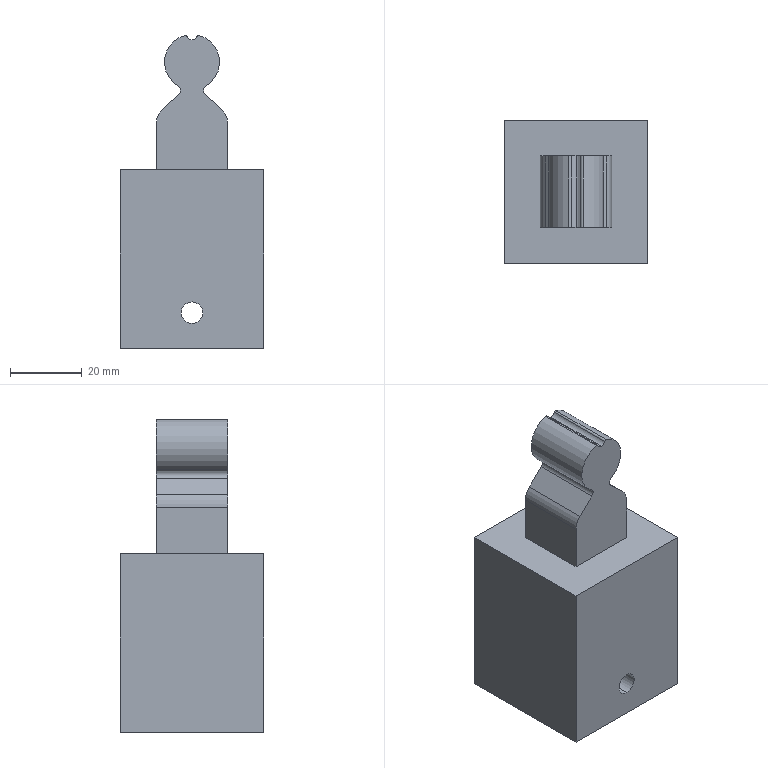Part | SolidWorks | features ICE 3, Extrusion 1 | 1 solid | 24 faces | box 40 x 40 x 87.456 mm | volume 90363 mm3 | cylinder 12 | plane 12 | commonest cylinder face diameters 3 x4 1 x2 6 x2 10 x2 15.4 x2
STEP:
#1=CARTESIAN_POINT('',(0.,30.,-18.));
#2=VERTEX_POINT('',#1);
#3=CARTESIAN_POINT('',(0.,30.,-12.));
#4=VERTEX_POINT('',#3);
#5=CARTESIAN_POINT('',(0.,30.,-15.));
#6=DIRECTION('',(0.,1.,0.));
#7=DIRECTION('',(0.,0.,1.));
#8=AXIS2_PLACEMENT_3D('',#5,#6,#7);
#9=CIRCLE('',#8,3.);
#10=EDGE_CURVE('',#2,#4,#9,.T.);
#11=ORIENTED_EDGE('',*,*,#10,.T.);
#12=CARTESIAN_POINT('',(0.,-10.,-12.));
#13=VERTEX_POINT('',#12);
#14=CARTESIAN_POINT('',(0.,49.,-12.));
#15=DIRECTION('',(0.,-1.,0.));
#16=VECTOR('',#15,1000.);
#17=LINE('',#14,#16);
#18=EDGE_CURVE('',#4,#13,#17,.T.);
#19=ORIENTED_EDGE('',*,*,#18,.T.);
#20=CARTESIAN_POINT('',(0.,-10.,-18.));
#21=VERTEX_POINT('',#20);
#22=CARTESIAN_POINT('',(0.,-10.,-15.));
#23=DIRECTION('',(0.,-1.,0.));
#24=DIRECTION('',(0.,0.,-1.));
#25=AXIS2_PLACEMENT_3D('',#22,#23,#24);
#26=CIRCLE('',#25,3.);
#27=EDGE_CURVE('',#13,#21,#26,.T.);
#28=ORIENTED_EDGE('',*,*,#27,.T.);
#29=CARTESIAN_POINT('',(0.,49.,-18.));
#30=DIRECTION('',(0.,-1.,0.));
#31=VECTOR('',#30,1000.);
#32=LINE('',#29,#31);
#33=EDGE_CURVE('',#2,#21,#32,.T.);
#34=ORIENTED_EDGE('',*,*,#33,.F.);
#35=EDGE_LOOP('',(#11,#19,#28,#34));
#36=FACE_OUTER_BOUND('',#35,.T.);
#37=CARTESIAN_POINT('',(0.,49.,-15.));
#38=DIRECTION('',(0.,-1.,0.));
#39=DIRECTION('',(0.,0.,-1.));
#40=AXIS2_PLACEMENT_3D('',#37,#38,#39);
#41=CYLINDRICAL_SURFACE('',#40,3.);
#42=ADVANCED_FACE('',(#36),#41,.F.);
#43=CARTESIAN_POINT('',(0.,20.,61.2));
#44=VERTEX_POINT('',#43);
#45=CARTESIAN_POINT('',(1.392,20.,62.142));
#46=VERTEX_POINT('',#45);
#47=CARTESIAN_POINT('',(0.,20.,62.7));
#48=DIRECTION('',(0.,-1.,0.));
#49=DIRECTION('',(0.,0.,1.));
#50=AXIS2_PLACEMENT_3D('',#47,#48,#49);
#51=CIRCLE('',#50,1.5);
#52=EDGE_CURVE('',#44,#46,#51,.T.);
#53=ORIENTED_EDGE('',*,*,#52,.F.);
#54=CARTESIAN_POINT('',(0.,0.,61.2));
#55=VERTEX_POINT('',#54);
#56=CARTESIAN_POINT('',(0.,20.,61.2));
#57=DIRECTION('',(0.,-1.,0.));
#58=VECTOR('',#57,1000.);
#59=LINE('',#56,#58);
#60=EDGE_CURVE('',#44,#55,#59,.T.);
#61=ORIENTED_EDGE('',*,*,#60,.T.);
#62=CARTESIAN_POINT('',(1.392,0.,62.142));
#63=VERTEX_POINT('',#62);
#64=CARTESIAN_POINT('',(0.,0.,62.7));
#65=DIRECTION('',(0.,-1.,0.));
#66=DIRECTION('',(0.,0.,1.));
#67=AXIS2_PLACEMENT_3D('',#64,#65,#66);
#68=CIRCLE('',#67,1.5);
#69=EDGE_CURVE('',#55,#63,#68,.T.);
#70=ORIENTED_EDGE('',*,*,#69,.T.);
#71=CARTESIAN_POINT('',(1.392,20.,62.142));
#72=DIRECTION('',(0.,-1.,0.));
#73=VECTOR('',#72,1000.);
#74=LINE('',#71,#73);
#75=EDGE_CURVE('',#46,#63,#74,.T.);
#76=ORIENTED_EDGE('',*,*,#75,.F.);
#77=EDGE_LOOP('',(#53,#61,#70,#76));
#78=FACE_OUTER_BOUND('',#77,.T.);
#79=CARTESIAN_POINT('',(0.,20.,62.7));
#80=DIRECTION('',(0.,-1.,0.));
#81=DIRECTION('',(0.,0.,-1.));
#82=AXIS2_PLACEMENT_3D('',#79,#80,#81);
#83=CYLINDRICAL_SURFACE('',#82,1.5);
#84=ADVANCED_FACE('',(#78),#83,.F.);
#85=CARTESIAN_POINT('',(10.,0.,25.));
#86=VERTEX_POINT('',#85);
#87=CARTESIAN_POINT('',(-10.,0.,25.));
#88=VERTEX_POINT('',#87);
#89=CARTESIAN_POINT('',(20.,0.,25.));
#90=DIRECTION('',(-1.,0.,0.));
#91=VECTOR('',#90,1000.);
#92=LINE('',#89,#91);
#93=EDGE_CURVE('',#86,#88,#92,.T.);
#94=ORIENTED_EDGE('',*,*,#93,.F.);
#95=CARTESIAN_POINT('',(10.,0.,37.869));
#96=VERTEX_POINT('',#95);
#97=CARTESIAN_POINT('',(10.,0.,25.));
#98=DIRECTION('',(0.,0.,-1.));
#99=VECTOR('',#98,1000.);
#100=LINE('',#97,#99);
#101=EDGE_CURVE('',#96,#86,#100,.T.);
#102=ORIENTED_EDGE('',*,*,#101,.F.);
#103=CARTESIAN_POINT('',(8.463,0.,41.476));
#104=VERTEX_POINT('',#103);
#105=CARTESIAN_POINT('',(5.,0.,37.869));
#106=DIRECTION('',(0.,1.,0.));
#107=DIRECTION('',(0.,0.,1.));
#108=AXIS2_PLACEMENT_3D('',#105,#106,#107);
#109=CIRCLE('',#108,5.);
#110=EDGE_CURVE('',#104,#96,#109,.T.);
#111=ORIENTED_EDGE('',*,*,#110,.F.);
#112=CARTESIAN_POINT('',(3.711,0.,46.039));
#113=VERTEX_POINT('',#112);
#114=CARTESIAN_POINT('',(8.463,0.,41.476));
#115=DIRECTION('',(0.7213,0.,-0.6926));
#116=VECTOR('',#115,1000.);
#117=LINE('',#114,#116);
#118=EDGE_CURVE('',#113,#104,#117,.T.);
#119=ORIENTED_EDGE('',*,*,#118,.F.);
#120=CARTESIAN_POINT('',(3.976,0.,48.406));
#121=VERTEX_POINT('',#120);
#122=CARTESIAN_POINT('',(4.75,0.,47.121));
#123=DIRECTION('',(0.,-1.,0.));
#124=DIRECTION('',(0.,0.,1.));
#125=AXIS2_PLACEMENT_3D('',#122,#123,#124);
#126=CIRCLE('',#125,1.5);
#127=EDGE_CURVE('',#121,#113,#126,.T.);
#128=ORIENTED_EDGE('',*,*,#127,.F.);
#129=CARTESIAN_POINT('',(1.986,0.,62.44));
#130=VERTEX_POINT('',#129);
#131=CARTESIAN_POINT('',(0.,0.,55.));
#132=DIRECTION('',(0.,1.,0.));
#133=DIRECTION('',(0.,0.,1.));
#134=AXIS2_PLACEMENT_3D('',#131,#132,#133);
#135=CIRCLE('',#134,7.7);
#136=EDGE_CURVE('',#130,#121,#135,.T.);
#137=ORIENTED_EDGE('',*,*,#136,.F.);
#138=CARTESIAN_POINT('',(1.857,0.,61.956));
#139=DIRECTION('',(0.,1.,0.));
#140=DIRECTION('',(0.,0.,1.));
#141=AXIS2_PLACEMENT_3D('',#138,#139,#140);
#142=CIRCLE('',#141,0.5);
#143=EDGE_CURVE('',#63,#130,#142,.T.);
#144=ORIENTED_EDGE('',*,*,#143,.F.);
#145=ORIENTED_EDGE('',*,*,#69,.F.);
#146=CARTESIAN_POINT('',(-1.392,0.,62.142));
#147=VERTEX_POINT('',#146);
#148=CARTESIAN_POINT('',(0.,0.,62.7));
#149=DIRECTION('',(0.,-1.,0.));
#150=DIRECTION('',(0.,0.,1.));
#151=AXIS2_PLACEMENT_3D('',#148,#149,#150);
#152=CIRCLE('',#151,1.5);
#153=EDGE_CURVE('',#147,#55,#152,.T.);
#154=ORIENTED_EDGE('',*,*,#153,.F.);
#155=CARTESIAN_POINT('',(-1.986,0.,62.44));
#156=VERTEX_POINT('',#155);
#157=CARTESIAN_POINT('',(-1.857,0.,61.956));
#158=DIRECTION('',(0.,1.,0.));
#159=DIRECTION('',(0.,0.,-1.));
#160=AXIS2_PLACEMENT_3D('',#157,#158,#159);
#161=CIRCLE('',#160,0.5);
#162=EDGE_CURVE('',#156,#147,#161,.T.);
#163=ORIENTED_EDGE('',*,*,#162,.F.);
#164=CARTESIAN_POINT('',(-3.976,0.,48.406));
#165=VERTEX_POINT('',#164);
#166=CARTESIAN_POINT('',(0.,0.,55.));
#167=DIRECTION('',(0.,1.,0.));
#168=DIRECTION('',(0.,0.,1.));
#169=AXIS2_PLACEMENT_3D('',#166,#167,#168);
#170=CIRCLE('',#169,7.7);
#171=EDGE_CURVE('',#165,#156,#170,.T.);
#172=ORIENTED_EDGE('',*,*,#171,.F.);
#173=CARTESIAN_POINT('',(-3.711,0.,46.039));
#174=VERTEX_POINT('',#173);
#175=CARTESIAN_POINT('',(-4.75,0.,47.121));
#176=DIRECTION('',(0.,-1.,0.));
#177=DIRECTION('',(0.,0.,1.));
#178=AXIS2_PLACEMENT_3D('',#175,#176,#177);
#179=CIRCLE('',#178,1.5);
#180=EDGE_CURVE('',#174,#165,#179,.T.);
#181=ORIENTED_EDGE('',*,*,#180,.F.);
#182=CARTESIAN_POINT('',(-8.463,0.,41.476));
#183=VERTEX_POINT('',#182);
#184=CARTESIAN_POINT('',(-8.463,0.,41.476));
#185=DIRECTION('',(0.7213,0.,0.6926));
#186=VECTOR('',#185,1000.);
#187=LINE('',#184,#186);
#188=EDGE_CURVE('',#183,#174,#187,.T.);
#189=ORIENTED_EDGE('',*,*,#188,.F.);
#190=CARTESIAN_POINT('',(-10.,0.,37.869));
#191=VERTEX_POINT('',#190);
#192=CARTESIAN_POINT('',(-5.,0.,37.869));
#193=DIRECTION('',(0.,1.,0.));
#194=DIRECTION('',(0.,0.,1.));
#195=AXIS2_PLACEMENT_3D('',#192,#193,#194);
#196=CIRCLE('',#195,5.);
#197=EDGE_CURVE('',#191,#183,#196,.T.);
#198=ORIENTED_EDGE('',*,*,#197,.F.);
#199=CARTESIAN_POINT('',(-10.,0.,25.));
#200=DIRECTION('',(0.,0.,1.));
#201=VECTOR('',#200,1000.);
#202=LINE('',#199,#201);
#203=EDGE_CURVE('',#88,#191,#202,.T.);
#204=ORIENTED_EDGE('',*,*,#203,.F.);
#205=EDGE_LOOP('',(#94,#102,#111,#119,#128,#137,#144,#145,#154,#163,#172,#181,#189,#198,#204));
#206=FACE_OUTER_BOUND('',#205,.T.);
#207=CARTESIAN_POINT('',(-5.,0.,37.869));
#208=DIRECTION('',(0.,1.,0.));
#209=DIRECTION('',(0.,0.,1.));
#210=AXIS2_PLACEMENT_3D('',#207,#208,#209);
#211=PLANE('',#210);
#212=ADVANCED_FACE('',(#206),#211,.F.);
#213=CARTESIAN_POINT('',(20.,30.,25.));
#214=VERTEX_POINT('',#213);
#215=CARTESIAN_POINT('',(20.,-10.,25.));
#216=VERTEX_POINT('',#215);
#217=CARTESIAN_POINT('',(20.,20.,25.));
#218=DIRECTION('',(0.,-1.,0.));
#219=VECTOR('',#218,1000.);
#220=LINE('',#217,#219);
#221=EDGE_CURVE('',#214,#216,#220,.T.);
#222=ORIENTED_EDGE('',*,*,#221,.T.);
#223=CARTESIAN_POINT('',(20.,-10.,-25.));
#224=VERTEX_POINT('',#223);
#225=CARTESIAN_POINT('',(20.,-10.,-25.));
#226=DIRECTION('',(0.,0.,1.));
#227=VECTOR('',#226,1000.);
#228=LINE('',#225,#227);
#229=EDGE_CURVE('',#224,#216,#228,.T.);
#230=ORIENTED_EDGE('',*,*,#229,.F.);
#231=CARTESIAN_POINT('',(20.,30.,-25.));
#232=VERTEX_POINT('',#231);
#233=CARTESIAN_POINT('',(20.,20.,-25.));
#234=DIRECTION('',(0.,-1.,0.));
#235=VECTOR('',#234,1000.);
#236=LINE('',#233,#235);
#237=EDGE_CURVE('',#232,#224,#236,.T.);
#238=ORIENTED_EDGE('',*,*,#237,.F.);
#239=CARTESIAN_POINT('',(20.,30.,-25.));
#240=DIRECTION('',(0.,0.,-1.));
#241=VECTOR('',#240,1000.);
#242=LINE('',#239,#241);
#243=EDGE_CURVE('',#214,#232,#242,.T.);
#244=ORIENTED_EDGE('',*,*,#243,.F.);
#245=EDGE_LOOP('',(#222,#230,#238,#244));
#246=FACE_OUTER_BOUND('',#245,.T.);
#247=CARTESIAN_POINT('',(20.,20.,25.));
#248=DIRECTION('',(-1.,0.,0.));
#249=DIRECTION('',(0.,0.,1.));
#250=AXIS2_PLACEMENT_3D('',#247,#248,#249);
#251=PLANE('',#250);
#252=ADVANCED_FACE('',(#246),#251,.F.);
#253=ORIENTED_EDGE('',*,*,#237,.T.);
#254=CARTESIAN_POINT('',(-20.,-10.,-25.));
#255=VERTEX_POINT('',#254);
#256=CARTESIAN_POINT('',(20.,-10.,-25.));
#257=DIRECTION('',(1.,0.,0.));
#258=VECTOR('',#257,1000.);
#259=LINE('',#256,#258);
#260=EDGE_CURVE('',#255,#224,#259,.T.);
#261=ORIENTED_EDGE('',*,*,#260,.F.);
#262=CARTESIAN_POINT('',(-20.,30.,-25.));
#263=VERTEX_POINT('',#262);
#264=CARTESIAN_POINT('',(-20.,20.,-25.));
#265=DIRECTION('',(0.,-1.,0.));
#266=VECTOR('',#265,1000.);
#267=LINE('',#264,#266);
#268=EDGE_CURVE('',#263,#255,#267,.T.);
#269=ORIENTED_EDGE('',*,*,#268,.F.);
#270=CARTESIAN_POINT('',(-20.,30.,-25.));
#271=DIRECTION('',(-1.,0.,0.));
#272=VECTOR('',#271,1000.);
#273=LINE('',#270,#272);
#274=EDGE_CURVE('',#232,#263,#273,.T.);
#275=ORIENTED_EDGE('',*,*,#274,.F.);
#276=EDGE_LOOP('',(#253,#261,#269,#275));
#277=FACE_OUTER_BOUND('',#276,.T.);
#278=CARTESIAN_POINT('',(-20.,20.,-25.));
#279=DIRECTION('',(0.,0.,1.));
#280=DIRECTION('',(1.,0.,0.));
#281=AXIS2_PLACEMENT_3D('',#278,#279,#280);
#282=PLANE('',#281);
#283=ADVANCED_FACE('',(#277),#282,.F.);
#284=ORIENTED_EDGE('',*,*,#268,.T.);
#285=CARTESIAN_POINT('',(-20.,-10.,25.));
#286=VERTEX_POINT('',#285);
#287=CARTESIAN_POINT('',(-20.,-10.,-25.));
#288=DIRECTION('',(0.,0.,-1.));
#289=VECTOR('',#288,1000.);
#290=LINE('',#287,#289);
#291=EDGE_CURVE('',#286,#255,#290,.T.);
#292=ORIENTED_EDGE('',*,*,#291,.F.);
#293=CARTESIAN_POINT('',(-20.,30.,25.));
#294=VERTEX_POINT('',#293);
#295=CARTESIAN_POINT('',(-20.,20.,25.));
#296=DIRECTION('',(0.,-1.,0.));
#297=VECTOR('',#296,1000.);
#298=LINE('',#295,#297);
#299=EDGE_CURVE('',#294,#286,#298,.T.);
#300=ORIENTED_EDGE('',*,*,#299,.F.);
#301=CARTESIAN_POINT('',(-20.,30.,-25.));
#302=DIRECTION('',(0.,0.,1.));
#303=VECTOR('',#302,1000.);
#304=LINE('',#301,#303);
#305=EDGE_CURVE('',#263,#294,#304,.T.);
#306=ORIENTED_EDGE('',*,*,#305,.F.);
#307=EDGE_LOOP('',(#284,#292,#300,#306));
#308=FACE_OUTER_BOUND('',#307,.T.);
#309=CARTESIAN_POINT('',(-20.,20.,25.));
#310=DIRECTION('',(1.,0.,0.));
#311=DIRECTION('',(0.,0.,-1.));
#312=AXIS2_PLACEMENT_3D('',#309,#310,#311);
#313=PLANE('',#312);
#314=ADVANCED_FACE('',(#308),#313,.F.);
#315=ORIENTED_EDGE('',*,*,#203,.T.);
#316=CARTESIAN_POINT('',(-10.,20.,37.869));
#317=VERTEX_POINT('',#316);
#318=CARTESIAN_POINT('',(-10.,20.,37.869));
#319=DIRECTION('',(0.,-1.,0.));
#320=VECTOR('',#319,1000.);
#321=LINE('',#318,#320);
#322=EDGE_CURVE('',#317,#191,#321,.T.);
#323=ORIENTED_EDGE('',*,*,#322,.F.);
#324=CARTESIAN_POINT('',(-10.,20.,25.));
#325=VERTEX_POINT('',#324);
#326=CARTESIAN_POINT('',(-10.,20.,25.));
#327=DIRECTION('',(0.,0.,1.));
#328=VECTOR('',#327,1000.);
#329=LINE('',#326,#328);
#330=EDGE_CURVE('',#325,#317,#329,.T.);
#331=ORIENTED_EDGE('',*,*,#330,.F.);
#332=CARTESIAN_POINT('',(-10.,20.,25.));
#333=DIRECTION('',(0.,-1.,0.));
#334=VECTOR('',#333,1000.);
#335=LINE('',#332,#334);
#336=EDGE_CURVE('',#325,#88,#335,.T.);
#337=ORIENTED_EDGE('',*,*,#336,.T.);
#338=EDGE_LOOP('',(#315,#323,#331,#337));
#339=FACE_OUTER_BOUND('',#338,.T.);
#340=CARTESIAN_POINT('',(-10.,20.,25.));
#341=DIRECTION('',(1.,0.,0.));
#342=DIRECTION('',(0.,0.,-1.));
#343=AXIS2_PLACEMENT_3D('',#340,#341,#342);
#344=PLANE('',#343);
#345=ADVANCED_FACE('',(#339),#344,.F.);
#346=ORIENTED_EDGE('',*,*,#197,.T.);
#347=CARTESIAN_POINT('',(-8.463,20.,41.476));
#348=VERTEX_POINT('',#347);
#349=CARTESIAN_POINT('',(-8.463,20.,41.476));
#350=DIRECTION('',(0.,-1.,0.));
#351=VECTOR('',#350,1000.);
#352=LINE('',#349,#351);
#353=EDGE_CURVE('',#348,#183,#352,.T.);
#354=ORIENTED_EDGE('',*,*,#353,.F.);
#355=CARTESIAN_POINT('',(-5.,20.,37.869));
#356=DIRECTION('',(0.,1.,0.));
#357=DIRECTION('',(0.,0.,1.));
#358=AXIS2_PLACEMENT_3D('',#355,#356,#357);
#359=CIRCLE('',#358,5.);
#360=EDGE_CURVE('',#317,#348,#359,.T.);
#361=ORIENTED_EDGE('',*,*,#360,.F.);
#362=ORIENTED_EDGE('',*,*,#322,.T.);
#363=EDGE_LOOP('',(#346,#354,#361,#362));
#364=FACE_OUTER_BOUND('',#363,.T.);
#365=CARTESIAN_POINT('',(-5.,20.,37.869));
#366=DIRECTION('',(0.,-1.,0.));
#367=DIRECTION('',(0.,0.,-1.));
#368=AXIS2_PLACEMENT_3D('',#365,#366,#367);
#369=CYLINDRICAL_SURFACE('',#368,5.);
#370=ADVANCED_FACE('',(#364),#369,.T.);
#371=ORIENTED_EDGE('',*,*,#188,.T.);
#372=CARTESIAN_POINT('',(-3.711,20.,46.039));
#373=VERTEX_POINT('',#372);
#374=CARTESIAN_POINT('',(-3.711,20.,46.039));
#375=DIRECTION('',(0.,-1.,0.));
#376=VECTOR('',#375,1000.);
#377=LINE('',#374,#376);
#378=EDGE_CURVE('',#373,#174,#377,.T.);
#379=ORIENTED_EDGE('',*,*,#378,.F.);
#380=CARTESIAN_POINT('',(-8.463,20.,41.476));
#381=DIRECTION('',(0.7213,0.,0.6926));
#382=VECTOR('',#381,1000.);
#383=LINE('',#380,#382);
#384=EDGE_CURVE('',#348,#373,#383,.T.);
#385=ORIENTED_EDGE('',*,*,#384,.F.);
#386=ORIENTED_EDGE('',*,*,#353,.T.);
#387=EDGE_LOOP('',(#371,#379,#385,#386));
#388=FACE_OUTER_BOUND('',#387,.T.);
#389=CARTESIAN_POINT('',(-8.463,20.,41.476));
#390=DIRECTION('',(0.6926,0.,-0.7213));
#391=DIRECTION('',(-0.7213,0.,-0.6926));
#392=AXIS2_PLACEMENT_3D('',#389,#390,#391);
#393=PLANE('',#392);
#394=ADVANCED_FACE('',(#388),#393,.F.);
#395=ORIENTED_EDGE('',*,*,#180,.T.);
#396=CARTESIAN_POINT('',(-3.976,20.,48.406));
#397=VERTEX_POINT('',#396);
#398=CARTESIAN_POINT('',(-3.976,20.,48.406));
#399=DIRECTION('',(0.,-1.,0.));
#400=VECTOR('',#399,1000.);
#401=LINE('',#398,#400);
#402=EDGE_CURVE('',#397,#165,#401,.T.);
#403=ORIENTED_EDGE('',*,*,#402,.F.);
#404=CARTESIAN_POINT('',(-4.75,20.,47.121));
#405=DIRECTION('',(0.,-1.,0.));
#406=DIRECTION('',(0.,0.,1.));
#407=AXIS2_PLACEMENT_3D('',#404,#405,#406);
#408=CIRCLE('',#407,1.5);
#409=EDGE_CURVE('',#373,#397,#408,.T.);
#410=ORIENTED_EDGE('',*,*,#409,.F.);
#411=ORIENTED_EDGE('',*,*,#378,.T.);
#412=EDGE_LOOP('',(#395,#403,#410,#411));
#413=FACE_OUTER_BOUND('',#412,.T.);
#414=CARTESIAN_POINT('',(-4.75,20.,47.121));
#415=DIRECTION('',(0.,-1.,0.));
#416=DIRECTION('',(0.,0.,-1.));
#417=AXIS2_PLACEMENT_3D('',#414,#415,#416);
#418=CYLINDRICAL_SURFACE('',#417,1.5);
#419=ADVANCED_FACE('',(#413),#418,.F.);
#420=ORIENTED_EDGE('',*,*,#171,.T.);
#421=CARTESIAN_POINT('',(-1.986,20.,62.44));
#422=VERTEX_POINT('',#421);
#423=CARTESIAN_POINT('',(-1.986,20.,62.44));
#424=DIRECTION('',(0.,-1.,0.));
#425=VECTOR('',#424,1000.);
#426=LINE('',#423,#425);
#427=EDGE_CURVE('',#422,#156,#426,.T.);
#428=ORIENTED_EDGE('',*,*,#427,.F.);
#429=CARTESIAN_POINT('',(0.,20.,55.));
#430=DIRECTION('',(0.,1.,0.));
#431=DIRECTION('',(0.,0.,1.));
#432=AXIS2_PLACEMENT_3D('',#429,#430,#431);
#433=CIRCLE('',#432,7.7);
#434=EDGE_CURVE('',#397,#422,#433,.T.);
#435=ORIENTED_EDGE('',*,*,#434,.F.);
#436=ORIENTED_EDGE('',*,*,#402,.T.);
#437=EDGE_LOOP('',(#420,#428,#435,#436));
#438=FACE_OUTER_BOUND('',#437,.T.);
#439=CARTESIAN_POINT('',(0.,20.,55.));
#440=DIRECTION('',(0.,-1.,0.));
#441=DIRECTION('',(0.,0.,-1.));
#442=AXIS2_PLACEMENT_3D('',#439,#440,#441);
#443=CYLINDRICAL_SURFACE('',#442,7.7);
#444=ADVANCED_FACE('',(#438),#443,.T.);
#445=ORIENTED_EDGE('',*,*,#162,.T.);
#446=CARTESIAN_POINT('',(-1.392,20.,62.142));
#447=VERTEX_POINT('',#446);
#448=CARTESIAN_POINT('',(-1.392,20.,62.142));
#449=DIRECTION('',(0.,-1.,0.));
#450=VECTOR('',#449,1000.);
#451=LINE('',#448,#450);
#452=EDGE_CURVE('',#447,#147,#451,.T.);
#453=ORIENTED_EDGE('',*,*,#452,.F.);
#454=CARTESIAN_POINT('',(-1.857,20.,61.956));
#455=DIRECTION('',(0.,1.,0.));
#456=DIRECTION('',(0.,0.,-1.));
#457=AXIS2_PLACEMENT_3D('',#454,#455,#456);
#458=CIRCLE('',#457,0.5);
#459=EDGE_CURVE('',#422,#447,#458,.T.);
#460=ORIENTED_EDGE('',*,*,#459,.F.);
#461=ORIENTED_EDGE('',*,*,#427,.T.);
#462=EDGE_LOOP('',(#445,#453,#460,#461));
#463=FACE_OUTER_BOUND('',#462,.T.);
#464=CARTESIAN_POINT('',(-1.857,20.,61.956));
#465=DIRECTION('',(0.,-1.,0.));
#466=DIRECTION('',(0.,0.,-1.));
#467=AXIS2_PLACEMENT_3D('',#464,#465,#466);
#468=CYLINDRICAL_SURFACE('',#467,0.5);
#469=ADVANCED_FACE('',(#463),#468,.T.);
#470=ORIENTED_EDGE('',*,*,#60,.F.);
#471=CARTESIAN_POINT('',(0.,20.,62.7));
#472=DIRECTION('',(0.,-1.,0.));
#473=DIRECTION('',(0.,0.,1.));
#474=AXIS2_PLACEMENT_3D('',#471,#472,#473);
#475=CIRCLE('',#474,1.5);
#476=EDGE_CURVE('',#447,#44,#475,.T.);
#477=ORIENTED_EDGE('',*,*,#476,.F.);
#478=ORIENTED_EDGE('',*,*,#452,.T.);
#479=ORIENTED_EDGE('',*,*,#153,.T.);
#480=EDGE_LOOP('',(#470,#477,#478,#479));
#481=FACE_OUTER_BOUND('',#480,.T.);
#482=CARTESIAN_POINT('',(0.,20.,62.7));
#483=DIRECTION('',(0.,-1.,0.));
#484=DIRECTION('',(0.,0.,-1.));
#485=AXIS2_PLACEMENT_3D('',#482,#483,#484);
#486=CYLINDRICAL_SURFACE('',#485,1.5);
#487=ADVANCED_FACE('',(#481),#486,.F.);
#488=ORIENTED_EDGE('',*,*,#143,.T.);
#489=CARTESIAN_POINT('',(1.986,20.,62.44));
#490=VERTEX_POINT('',#489);
#491=CARTESIAN_POINT('',(1.986,20.,62.44));
#492=DIRECTION('',(0.,-1.,0.));
#493=VECTOR('',#492,1000.);
#494=LINE('',#491,#493);
#495=EDGE_CURVE('',#490,#130,#494,.T.);
#496=ORIENTED_EDGE('',*,*,#495,.F.);
#497=CARTESIAN_POINT('',(1.857,20.,61.956));
#498=DIRECTION('',(0.,1.,0.));
#499=DIRECTION('',(0.,0.,1.));
#500=AXIS2_PLACEMENT_3D('',#497,#498,#499);
#501=CIRCLE('',#500,0.5);
#502=EDGE_CURVE('',#46,#490,#501,.T.);
#503=ORIENTED_EDGE('',*,*,#502,.F.);
#504=ORIENTED_EDGE('',*,*,#75,.T.);
#505=EDGE_LOOP('',(#488,#496,#503,#504));
#506=FACE_OUTER_BOUND('',#505,.T.);
#507=CARTESIAN_POINT('',(1.857,20.,61.956));
#508=DIRECTION('',(0.,-1.,0.));
#509=DIRECTION('',(0.,0.,-1.));
#510=AXIS2_PLACEMENT_3D('',#507,#508,#509);
#511=CYLINDRICAL_SURFACE('',#510,0.5);
#512=ADVANCED_FACE('',(#506),#511,.T.);
#513=ORIENTED_EDGE('',*,*,#136,.T.);
#514=CARTESIAN_POINT('',(3.976,20.,48.406));
#515=VERTEX_POINT('',#514);
#516=CARTESIAN_POINT('',(3.976,20.,48.406));
#517=DIRECTION('',(0.,-1.,0.));
#518=VECTOR('',#517,1000.);
#519=LINE('',#516,#518);
#520=EDGE_CURVE('',#515,#121,#519,.T.);
#521=ORIENTED_EDGE('',*,*,#520,.F.);
#522=CARTESIAN_POINT('',(0.,20.,55.));
#523=DIRECTION('',(0.,1.,0.));
#524=DIRECTION('',(0.,0.,1.));
#525=AXIS2_PLACEMENT_3D('',#522,#523,#524);
#526=CIRCLE('',#525,7.7);
#527=EDGE_CURVE('',#490,#515,#526,.T.);
#528=ORIENTED_EDGE('',*,*,#527,.F.);
#529=ORIENTED_EDGE('',*,*,#495,.T.);
#530=EDGE_LOOP('',(#513,#521,#528,#529));
#531=FACE_OUTER_BOUND('',#530,.T.);
#532=CARTESIAN_POINT('',(0.,20.,55.));
#533=DIRECTION('',(0.,-1.,0.));
#534=DIRECTION('',(0.,0.,-1.));
#535=AXIS2_PLACEMENT_3D('',#532,#533,#534);
#536=CYLINDRICAL_SURFACE('',#535,7.7);
#537=ADVANCED_FACE('',(#531),#536,.T.);
#538=ORIENTED_EDGE('',*,*,#127,.T.);
#539=CARTESIAN_POINT('',(3.711,20.,46.039));
#540=VERTEX_POINT('',#539);
#541=CARTESIAN_POINT('',(3.711,20.,46.039));
#542=DIRECTION('',(0.,-1.,0.));
#543=VECTOR('',#542,1000.);
#544=LINE('',#541,#543);
#545=EDGE_CURVE('',#540,#113,#544,.T.);
#546=ORIENTED_EDGE('',*,*,#545,.F.);
#547=CARTESIAN_POINT('',(4.75,20.,47.121));
#548=DIRECTION('',(0.,-1.,0.));
#549=DIRECTION('',(0.,0.,1.));
#550=AXIS2_PLACEMENT_3D('',#547,#548,#549);
#551=CIRCLE('',#550,1.5);
#552=EDGE_CURVE('',#515,#540,#551,.T.);
#553=ORIENTED_EDGE('',*,*,#552,.F.);
#554=ORIENTED_EDGE('',*,*,#520,.T.);
#555=EDGE_LOOP('',(#538,#546,#553,#554));
#556=FACE_OUTER_BOUND('',#555,.T.);
#557=CARTESIAN_POINT('',(4.75,20.,47.121));
#558=DIRECTION('',(0.,-1.,0.));
#559=DIRECTION('',(0.,0.,-1.));
#560=AXIS2_PLACEMENT_3D('',#557,#558,#559);
#561=CYLINDRICAL_SURFACE('',#560,1.5);
#562=ADVANCED_FACE('',(#556),#561,.F.);
#563=ORIENTED_EDGE('',*,*,#118,.T.);
#564=CARTESIAN_POINT('',(8.463,20.,41.476));
#565=VERTEX_POINT('',#564);
#566=CARTESIAN_POINT('',(8.463,20.,41.476));
#567=DIRECTION('',(0.,-1.,0.));
#568=VECTOR('',#567,1000.);
#569=LINE('',#566,#568);
#570=EDGE_CURVE('',#565,#104,#569,.T.);
#571=ORIENTED_EDGE('',*,*,#570,.F.);
#572=CARTESIAN_POINT('',(8.463,20.,41.476));
#573=DIRECTION('',(0.7213,0.,-0.6926));
#574=VECTOR('',#573,1000.);
#575=LINE('',#572,#574);
#576=EDGE_CURVE('',#540,#565,#575,.T.);
#577=ORIENTED_EDGE('',*,*,#576,.F.);
#578=ORIENTED_EDGE('',*,*,#545,.T.);
#579=EDGE_LOOP('',(#563,#571,#577,#578));
#580=FACE_OUTER_BOUND('',#579,.T.);
#581=CARTESIAN_POINT('',(8.463,20.,41.476));
#582=DIRECTION('',(-0.6926,0.,-0.7213));
#583=DIRECTION('',(-0.7213,0.,0.6926));
#584=AXIS2_PLACEMENT_3D('',#581,#582,#583);
#585=PLANE('',#584);
#586=ADVANCED_FACE('',(#580),#585,.F.);
#587=ORIENTED_EDGE('',*,*,#110,.T.);
#588=CARTESIAN_POINT('',(10.,20.,37.869));
#589=VERTEX_POINT('',#588);
#590=CARTESIAN_POINT('',(10.,20.,37.869));
#591=DIRECTION('',(0.,-1.,0.));
#592=VECTOR('',#591,1000.);
#593=LINE('',#590,#592);
#594=EDGE_CURVE('',#589,#96,#593,.T.);
#595=ORIENTED_EDGE('',*,*,#594,.F.);
#596=CARTESIAN_POINT('',(5.,20.,37.869));
#597=DIRECTION('',(0.,1.,0.));
#598=DIRECTION('',(0.,0.,1.));
#599=AXIS2_PLACEMENT_3D('',#596,#597,#598);
#600=CIRCLE('',#599,5.);
#601=EDGE_CURVE('',#565,#589,#600,.T.);
#602=ORIENTED_EDGE('',*,*,#601,.F.);
#603=ORIENTED_EDGE('',*,*,#570,.T.);
#604=EDGE_LOOP('',(#587,#595,#602,#603));
#605=FACE_OUTER_BOUND('',#604,.T.);
#606=CARTESIAN_POINT('',(5.,20.,37.869));
#607=DIRECTION('',(0.,-1.,0.));
#608=DIRECTION('',(0.,0.,-1.));
#609=AXIS2_PLACEMENT_3D('',#606,#607,#608);
#610=CYLINDRICAL_SURFACE('',#609,5.);
#611=ADVANCED_FACE('',(#605),#610,.T.);
#612=ORIENTED_EDGE('',*,*,#101,.T.);
#613=CARTESIAN_POINT('',(10.,20.,25.));
#614=VERTEX_POINT('',#613);
#615=CARTESIAN_POINT('',(10.,20.,25.));
#616=DIRECTION('',(0.,-1.,0.));
#617=VECTOR('',#616,1000.);
#618=LINE('',#615,#617);
#619=EDGE_CURVE('',#614,#86,#618,.T.);
#620=ORIENTED_EDGE('',*,*,#619,.F.);
#621=CARTESIAN_POINT('',(10.,20.,25.));
#622=DIRECTION('',(0.,0.,-1.));
#623=VECTOR('',#622,1000.);
#624=LINE('',#621,#623);
#625=EDGE_CURVE('',#589,#614,#624,.T.);
#626=ORIENTED_EDGE('',*,*,#625,.F.);
#627=ORIENTED_EDGE('',*,*,#594,.T.);
#628=EDGE_LOOP('',(#612,#620,#626,#627));
#629=FACE_OUTER_BOUND('',#628,.T.);
#630=CARTESIAN_POINT('',(10.,20.,25.));
#631=DIRECTION('',(-1.,0.,0.));
#632=DIRECTION('',(0.,0.,1.));
#633=AXIS2_PLACEMENT_3D('',#630,#631,#632);
#634=PLANE('',#633);
#635=ADVANCED_FACE('',(#629),#634,.F.);
#636=CARTESIAN_POINT('',(20.,-10.,25.));
#637=DIRECTION('',(-1.,0.,0.));
#638=VECTOR('',#637,1000.);
#639=LINE('',#636,#638);
#640=EDGE_CURVE('',#216,#286,#639,.T.);
#641=ORIENTED_EDGE('',*,*,#640,.F.);
#642=ORIENTED_EDGE('',*,*,#221,.F.);
#643=CARTESIAN_POINT('',(-20.,30.,25.));
#644=DIRECTION('',(1.,0.,0.));
#645=VECTOR('',#644,1000.);
#646=LINE('',#643,#645);
#647=EDGE_CURVE('',#294,#214,#646,.T.);
#648=ORIENTED_EDGE('',*,*,#647,.F.);
#649=ORIENTED_EDGE('',*,*,#299,.T.);
#650=EDGE_LOOP('',(#641,#642,#648,#649));
#651=FACE_OUTER_BOUND('',#650,.T.);
#652=ORIENTED_EDGE('',*,*,#619,.T.);
#653=ORIENTED_EDGE('',*,*,#93,.T.);
#654=ORIENTED_EDGE('',*,*,#336,.F.);
#655=CARTESIAN_POINT('',(-20.,20.,25.));
#656=DIRECTION('',(1.,0.,0.));
#657=VECTOR('',#656,1000.);
#658=LINE('',#655,#657);
#659=EDGE_CURVE('',#325,#614,#658,.T.);
#660=ORIENTED_EDGE('',*,*,#659,.T.);
#661=EDGE_LOOP('',(#652,#653,#654,#660));
#662=FACE_BOUND('',#661,.T.);
#663=CARTESIAN_POINT('',(10.,20.,25.));
#664=DIRECTION('',(0.,0.,-1.));
#665=DIRECTION('',(-1.,0.,0.));
#666=AXIS2_PLACEMENT_3D('',#663,#664,#665);
#667=PLANE('',#666);
#668=ADVANCED_FACE('',(#651,#662),#667,.F.);
#669=ORIENTED_EDGE('',*,*,#659,.F.);
#670=ORIENTED_EDGE('',*,*,#330,.T.);
#671=ORIENTED_EDGE('',*,*,#360,.T.);
#672=ORIENTED_EDGE('',*,*,#384,.T.);
#673=ORIENTED_EDGE('',*,*,#409,.T.);
#674=ORIENTED_EDGE('',*,*,#434,.T.);
#675=ORIENTED_EDGE('',*,*,#459,.T.);
#676=ORIENTED_EDGE('',*,*,#476,.T.);
#677=ORIENTED_EDGE('',*,*,#52,.T.);
#678=ORIENTED_EDGE('',*,*,#502,.T.);
#679=ORIENTED_EDGE('',*,*,#527,.T.);
#680=ORIENTED_EDGE('',*,*,#552,.T.);
#681=ORIENTED_EDGE('',*,*,#576,.T.);
#682=ORIENTED_EDGE('',*,*,#601,.T.);
#683=ORIENTED_EDGE('',*,*,#625,.T.);
#684=EDGE_LOOP('',(#669,#670,#671,#672,#673,#674,#675,#676,#677,#678,#679,#680,#681,#682,#683));
#685=FACE_OUTER_BOUND('',#684,.T.);
#686=CARTESIAN_POINT('',(-5.,20.,37.869));
#687=DIRECTION('',(0.,1.,0.));
#688=DIRECTION('',(0.,0.,1.));
#689=AXIS2_PLACEMENT_3D('',#686,#687,#688);
#690=PLANE('',#689);
#691=ADVANCED_FACE('',(#685),#690,.T.);
#692=ORIENTED_EDGE('',*,*,#10,.F.);
#693=CARTESIAN_POINT('',(0.,30.,-15.));
#694=DIRECTION('',(0.,1.,0.));
#695=DIRECTION('',(0.,0.,1.));
#696=AXIS2_PLACEMENT_3D('',#693,#694,#695);
#697=CIRCLE('',#696,3.);
#698=EDGE_CURVE('',#4,#2,#697,.T.);
#699=ORIENTED_EDGE('',*,*,#698,.F.);
#700=EDGE_LOOP('',(#692,#699));
#701=FACE_BOUND('',#700,.T.);
#702=ORIENTED_EDGE('',*,*,#305,.T.);
#703=ORIENTED_EDGE('',*,*,#647,.T.);
#704=ORIENTED_EDGE('',*,*,#243,.T.);
#705=ORIENTED_EDGE('',*,*,#274,.T.);
#706=EDGE_LOOP('',(#702,#703,#704,#705));
#707=FACE_OUTER_BOUND('',#706,.T.);
#708=CARTESIAN_POINT('',(0.,30.,0.));
#709=DIRECTION('',(0.,1.,0.));
#710=DIRECTION('',(0.,0.,1.));
#711=AXIS2_PLACEMENT_3D('',#708,#709,#710);
#712=PLANE('',#711);
#713=ADVANCED_FACE('',(#701,#707),#712,.T.);
#714=CARTESIAN_POINT('',(0.,-10.,-15.));
#715=DIRECTION('',(0.,-1.,0.));
#716=DIRECTION('',(0.,0.,-1.));
#717=AXIS2_PLACEMENT_3D('',#714,#715,#716);
#718=CIRCLE('',#717,3.);
#719=EDGE_CURVE('',#21,#13,#718,.T.);
#720=ORIENTED_EDGE('',*,*,#719,.F.);
#721=ORIENTED_EDGE('',*,*,#27,.F.);
#722=EDGE_LOOP('',(#720,#721));
#723=FACE_BOUND('',#722,.T.);
#724=ORIENTED_EDGE('',*,*,#229,.T.);
#725=ORIENTED_EDGE('',*,*,#640,.T.);
#726=ORIENTED_EDGE('',*,*,#291,.T.);
#727=ORIENTED_EDGE('',*,*,#260,.T.);
#728=EDGE_LOOP('',(#724,#725,#726,#727));
#729=FACE_OUTER_BOUND('',#728,.T.);
#730=CARTESIAN_POINT('',(0.,-10.,0.));
#731=DIRECTION('',(0.,-1.,0.));
#732=DIRECTION('',(0.,0.,-1.));
#733=AXIS2_PLACEMENT_3D('',#730,#731,#732);
#734=PLANE('',#733);
#735=ADVANCED_FACE('',(#723,#729),#734,.T.);
#736=ORIENTED_EDGE('',*,*,#18,.F.);
#737=ORIENTED_EDGE('',*,*,#698,.T.);
#738=ORIENTED_EDGE('',*,*,#33,.T.);
#739=ORIENTED_EDGE('',*,*,#719,.T.);
#740=EDGE_LOOP('',(#736,#737,#738,#739));
#741=FACE_OUTER_BOUND('',#740,.T.);
#742=CARTESIAN_POINT('',(0.,49.,-15.));
#743=DIRECTION('',(0.,-1.,0.));
#744=DIRECTION('',(0.,0.,-1.));
#745=AXIS2_PLACEMENT_3D('',#742,#743,#744);
#746=CYLINDRICAL_SURFACE('',#745,3.);
#747=ADVANCED_FACE('',(#741),#746,.F.);
#748=CLOSED_SHELL('',(#42,#84,#212,#252,#283,#314,#345,#370,#394,#419,#444,#469,#487,#512,#537,#562,#586,#611,#635,#668,#691,#713,#735,#747));
#749=MANIFOLD_SOLID_BREP('',#748);
#750=CARTESIAN_POINT('',(0.,0.,0.));
#751=DIRECTION('',(0.,0.,1.));
#752=DIRECTION('',(1.,0.,0.));
#753=AXIS2_PLACEMENT_3D('',#750,#751,#752);
#754=(LENGTH_UNIT()NAMED_UNIT(*)SI_UNIT(.MILLI.,.METRE.));
#755=UNCERTAINTY_MEASURE_WITH_UNIT(LENGTH_MEASURE(0.00001),#754,'','');
#756=(NAMED_UNIT(*)PLANE_ANGLE_UNIT()SI_UNIT($,.RADIAN.));
#757=(NAMED_UNIT(*)SI_UNIT($,.STERADIAN.)SOLID_ANGLE_UNIT());
#758=(GEOMETRIC_REPRESENTATION_CONTEXT(3)GLOBAL_UNCERTAINTY_ASSIGNED_CONTEXT((#755))GLOBAL_UNIT_ASSIGNED_CONTEXT((#754,#756,#757))REPRESENTATION_CONTEXT('',''));
#759=ADVANCED_BREP_SHAPE_REPRESENTATION('',(#749,#753),#758);